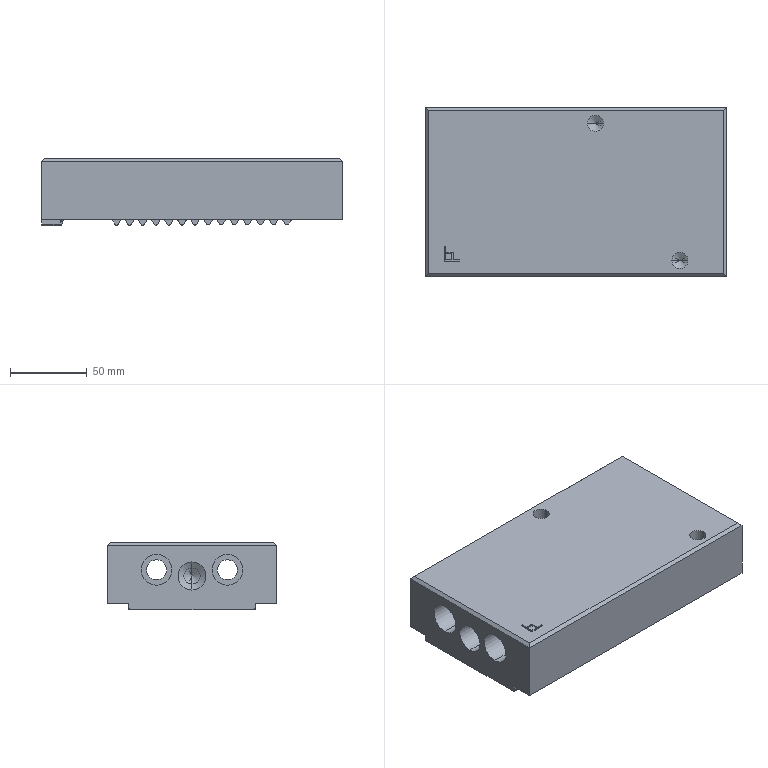Part | SolidWorks | features BaseBody 1 | 1 solid | 233 faces | box 195 x 110 x 44 mm | volume 788645 mm3 | plane 139 | cylinder 80 | cone 10 | sphere 2 | torus 2 | commonest cylinder face diameters 2 x56 2.4 x6 10.5 x4 13 x4 20 x4 10.7 x2